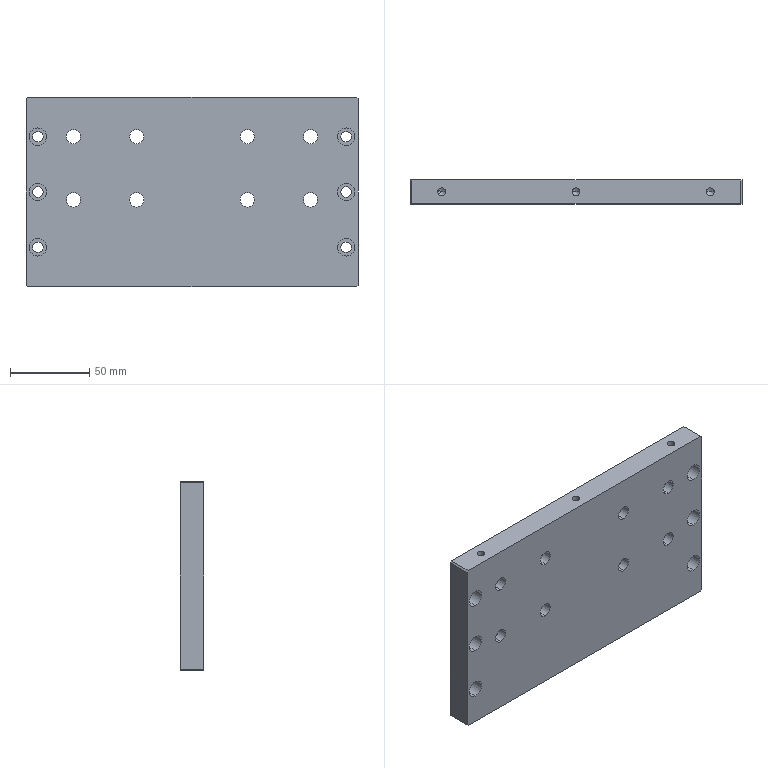Part | SolidWorks | features BaseBody 1 | 1 solid | 108 faces | box 210 x 15 x 120 mm | volume 353946 mm3 | cylinder 70 | plane 24 | cone 14 | commonest cylinder face diameters 9 x16 15 x16 5 x14 6.6 x12 11 x12